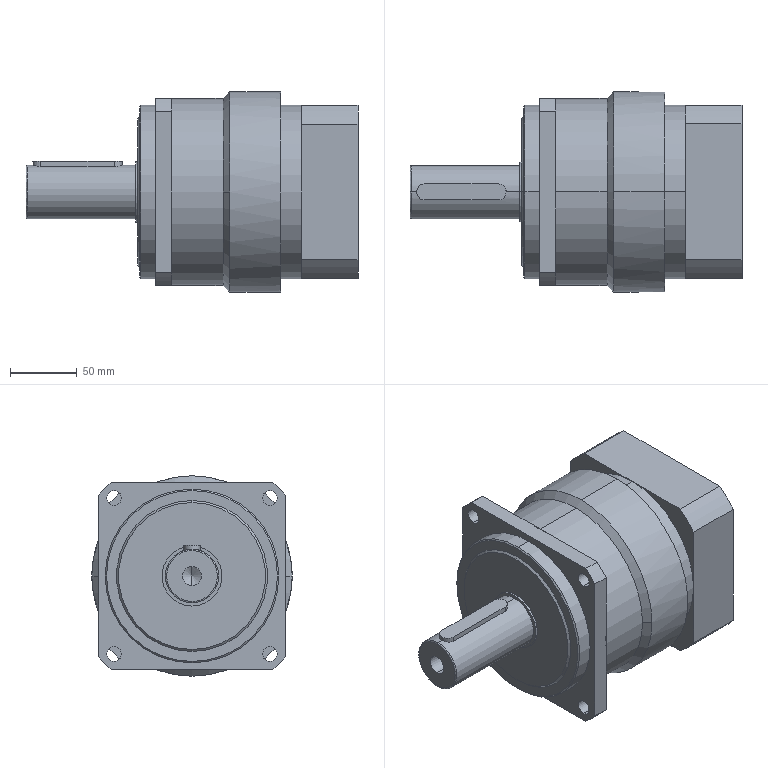Part | SolidWorks | features BaseBody 1 | 1 solid | 94 faces | box 248.5 x 150 x 150 mm | volume 2601531 mm3 | cylinder 47 | plane 29 | cone 16 | spline 2 | commonest cylinder face diameters 6.8 x8 11 x8 130 x4 165 x4 185 x4 12 x3